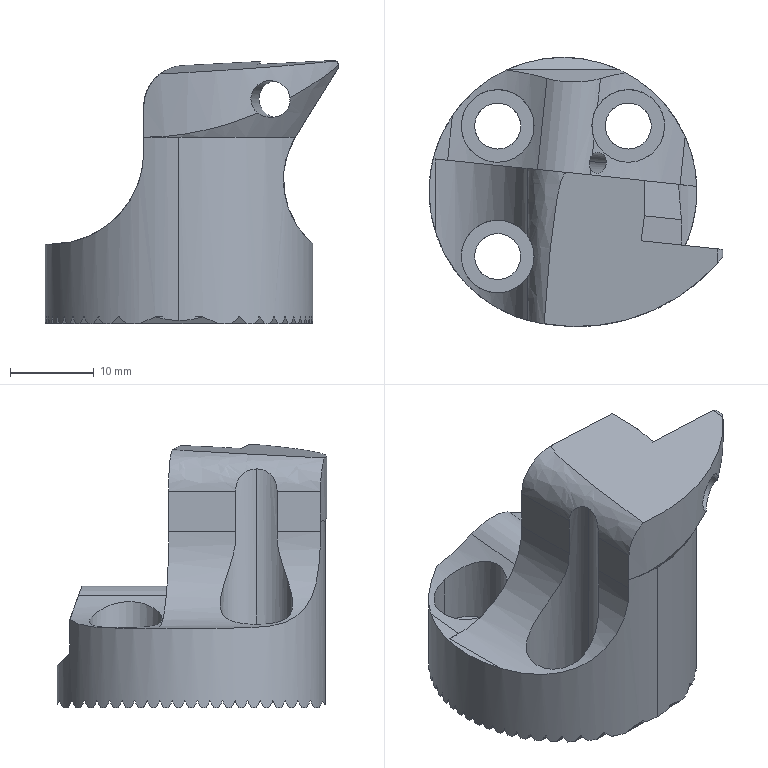Part | 1 solid | 176 faces | volume 11802 mm3 | plane 139 | cylinder 31 | cone 5 | spline 1 | commonest cylinder face diameters 5.5 x6 8.7 x6 32 x3 2.5 x2 4.4 x2 10.5 x2